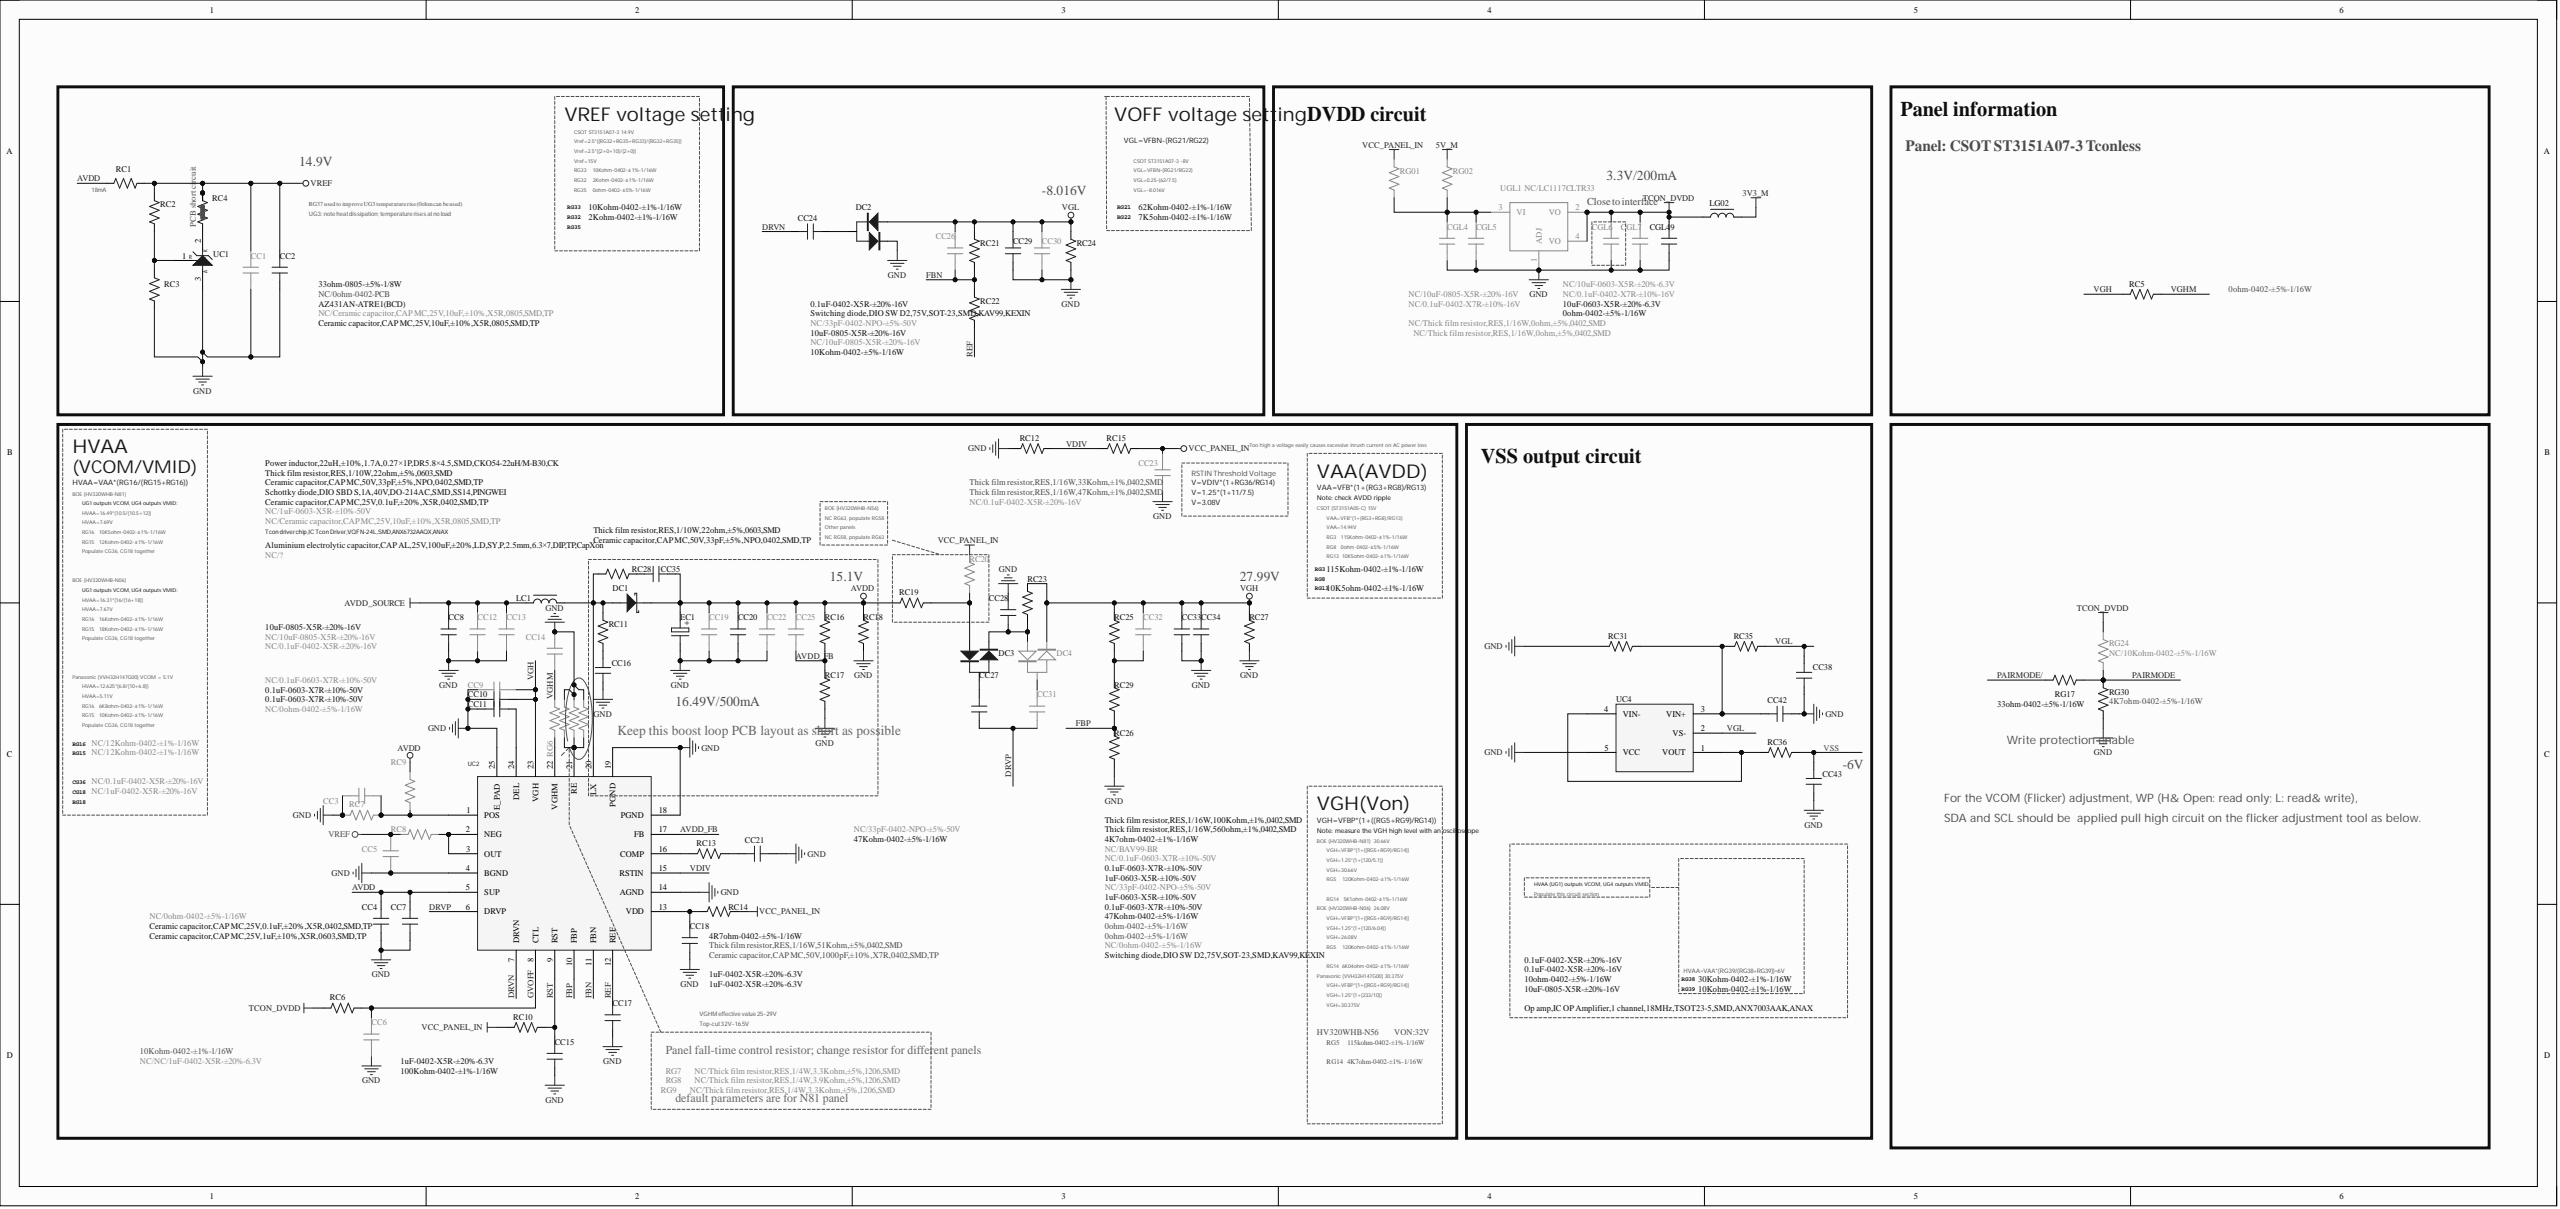Circuit board | Altium Designer | 951 parts | 509 nets | one sheet of the schematic
Parts on this sheet (reference | value | footprint):
CC1 | NC/Ceramic capacitor,CAP MC,25V,10uF,±10%,X5R,0805,SMD,TP | C0805
CC2 | Ceramic capacitor,CAP MC,25V,10uF,±10%,X5R,0805,SMD,TP | C0805
CC3 | NC/0.1uF-0402-X5R-±20%-16V | C0402
CC4 | Ceramic capacitor,CAP MC,25V,1uF,±10%,X5R,0603,SMD,TP | C0603
CC5 | NC/1uF-0402-X5R-±20%-16V | C0402
CC6 | NC/NC/1uF-0402-X5R-±20%-6.3V | C0402
CC7 | Ceramic capacitor,CAP MC,25V,0.1uF,±20%,X5R,0402,SMD,TP | C0402
CC8 | 10uF-0805-X5R-±20%-16V | C0805
CC9 | NC/0.1uF-0603-X7R-±10%-50V | C0603
CC10 | 0.1uF-0603-X7R-±10%-50V | C0603
CC11 | 0.1uF-0603-X7R-±10%-50V | C0603
CC12 | NC/10uF-0805-X5R-±20%-16V | C0805
CC13 | NC/0.1uF-0402-X5R-±20%-16V | C0402
CC14 | NC/? | C0805
CC15 | 1uF-0402-X5R-±20%-6.3V | C0402
CC16 | Ceramic capacitor,CAP MC,50V,33pF,±5%,NPO,0402,SMD,TP | C0402
CC17 | 1uF-0402-X5R-±20%-6.3V | C0402
CC18 | 1uF-0402-X5R-±20%-6.3V | C0402
CC19 | NC/Ceramic capacitor,CAP MC,25V,10uF,±10%,X5R,0805,SMD,TP | C0805
CC20 | Ceramic capacitor,CAP MC,25V,0.1uF,±20%,X5R,0402,SMD,TP | C0402
CC21 | Ceramic capacitor,CAP MC,50V,1000pF,±10%,X7R,0402,SMD,TP | C0402
CC22 | NC/1uF-0603-X5R-±10%-50V | C0603
CC23 | NC/0.1uF-0402-X5R-±20%-16V | C0402
CC24 | 0.1uF-0402-X5R-±20%-16V | C0402
CC25 | NC/33pF-0402-NPO-±5%-50V | C0402
CC26 | NC/33pF-0402-NPO-±5%-50V | C0402
CC27 | 0.1uF-0603-X7R-±10%-50V | C0603
CC28 | 1uF-0603-X5R-±10%-50V | C0603
CC29 | 10uF-0805-X5R-±20%-16V | C0805
CC30 | NC/10uF-0805-X5R-±20%-16V | C0805
CC31 | NC/0.1uF-0603-X7R-±10%-50V | C0603
CC32 | NC/33pF-0402-NPO-±5%-50V | C0402
CC33 | 1uF-0603-X5R-±10%-50V | C0603
CC34 | 0.1uF-0603-X7R-±10%-50V | C0603
CC35 | Ceramic capacitor,CAP MC,50V,33pF,±5%,NPO,0402,SMD,TP | C0402
CC38 | 0.1uF-0402-X5R-±20%-16V | C0402
CC42 | 0.1uF-0402-X5R-±20%-16V | C0402
CC43 | 10uF-0805-X5R-±20%-16V | C0805
CGL4 | NC/10uF-0805-X5R-±20%-16V | C0805
CGL5 | NC/0.1uF-0402-X7R-±10%-16V | C0402
CGL6 | NC/10uF-0603-X5R-±20%-6.3V | C0603
CGL7 | NC/0.1uF-0402-X7R-±10%-16V | C0402
CGL49 | 10uF-0603-X5R-±20%-6.3V | C0603
DC1 | Schottky diode,DIO SBD S,1A,40V,DO-214AC,SMD,SS14,PINGWEI | DIODE-S-1
DC2 | Switching diode,DIO SW D2,75V,SOT-23,SMD,KAV99,KEXIN | SO-23
DC3 | Switching diode,DIO SW D2,75V,SOT-23,SMD,KAV99,KEXIN | SO-23
DC4 | NC/BAV99-BR | SO-23
LG02 | 0ohm-0402-±5%-1/16W | L0402
RC1 | 33ohm-0805-±5%-1/8W | R0805
RC2 | 10Kohm-0402-±1%-1/16W | R0402
RC3 | 2Kohm-0402-±1%-1/16W | R0402
RC4 | NC/0ohm-0402-PCB | R0402SC
RC5 | 0ohm-0402-±5%-1/16W | R0402
RC6 | 10Kohm-0402-±1%-1/16W | R0402
RC7 | NC/12Kohm-0402-±1%-1/16W | R0402
RC8 | NC/0ohm-0402-±5%-1/16W | R0402
RC9 | NC/12Kohm-0402-±1%-1/16W | R0402
RC10 | 100Kohm-0402-±1%-1/16W | R0402
RC11 | Thick film resistor,RES,1/10W,22ohm,±5%,0603,SMD | R0603
RC12 | Thick film resistor,RES,1/16W,33Kohm,±1%,0402,SMD | R0402
RC13 | Thick film resistor,RES,1/16W,51Kohm,±5%,0402,SMD | R0402
RC14 | 4R7ohm-0402-±5%-1/16W | R0402
RC15 | Thick film resistor,RES,1/16W,47Kohm,±1%,0402,SMD | R0402
RC16 | 115Kohm-0402-±1%-1/16W | R0402
RC17 | 10K5ohm-0402-±1%-1/16W | R0402
RC18 | 47Kohm-0402-±5%-1/16W | R0402
RC19 | 0ohm-0402-±5%-1/16W | R0402
RC20 | NC/0ohm-0402-±5%-1/16W | R0402
RC21 | 62Kohm-0402-±1%-1/16W | R0402
RC22 | 7K5ohm-0402-±1%-1/16W | R0402
RC23 | 0ohm-0402-±5%-1/16W | R0402
RC24 | 10Kohm-0402-±5%-1/16W | R0402
RC25 | Thick film resistor,RES,1/16W,100Kohm,±1%,0402,SMD | R0402
RC26 | 4K7ohm-0402-±1%-1/16W | R0402
RC27 | 47Kohm-0402-±5%-1/16W | R0402
RC28 | Thick film resistor,RES,1/10W,22ohm,±5%,0603,SMD | R0603
RC29 | Thick film resistor,RES,1/16W,560ohm,±1%,0402,SMD | R0402
RC31 | 30Kohm-0402-±1%-1/16W | R0402
RC35 | 10Kohm-0402-±1%-1/16W | R0402
RC36 | 10ohm-0402-±5%-1/16W | R0402
RG01 | NC/Thick film resistor,RES,1/16W,0ohm,±5%,0402,SMD | R0402
RG02 | NC/Thick film resistor,RES,1/16W,0ohm,±5%,0402,SMD | R0402
RG6 | NC/0ohm-0402-±5%-1/16W | R0402
RG7 | NC/Thick film resistor,RES,1/4W,3.3Kohm,±5%,1206,SMD | R1206
RG8 | NC/Thick film resistor,RES,1/4W,3.9Kohm,±5%,1206,SMD | R1206
RG9 | NC/Thick film resistor,RES,1/4W,3.3Kohm,±5%,1206,SMD | R1206
RG17 | 33ohm-0402-±5%-1/16W | R0402
RG24 | NC/10Kohm-0402-±5%-1/16W | R0402
RG30 | 4K7ohm-0402-±5%-1/16W | R0402
UC1 | AZ431AN-ATRE1(BCD) | SO-23-1
UC2 | Tcon driver chip,IC Tcon Driver,VQFN-24L,SMD,ANX6732AAQX,ANAX | QFN24/0.5-5
UC4 | Op amp,IC OP Amplifier,1 channel,18MHz,TSOT23-5,SMD,ANX7003AAK,ANAX | SOT-23-5
UGL1 | NC/LC1117CLTR33 | SOT-223
Nets of these parts (net: part-pin ...):
VSS: CC43-2 RC36-2
VREF: CC1-2 CC2-2 CC5-1 RC1-2 RC2-2 RC4-2 RC4-3 RC8-1
VGL: CC26-2 CC29-1 CC30-1 CC38-1 DC2-1 RC21-2 RC24-2 RC35-2 UC4-2
VGHM: CC14-2 RC5-1 RG6-2
VGH: CC9-1 CC10-1 CC32-2 CC33-2 CC34-2 DC4-3 RC5-2 RC23-2 RC25-2 RC27-2 UC2-23
VDIV: RC12-2 RC15-1 UC2-15
VCC_PANEL_IN: CC23-2 RC10-2 RC14-2 RC15-2 RC20-1 RG01-2
TCON_DVDD: CGL6-1 CGL7-1 CGL49-1 LG02-1 RC6-2 RG24-1 UGL1-2 UGL1-4
RST: CC15-2 RC10-1 UC2-9
REF: CC17-2 RC22-1 UC2-12
PAIRMODE/: RG17-1
PAIRMODE: RG17-2 RG24-2 RG30-1
NetRG7_1: RG7-1 RG8-1 RG9-1 UC2-21
NetRG6_1: RG6-1 UC2-22
NetRC36_1: RC36-1 UC4-1 UC4-4
NetRC13_1: RC13-1 UC2-16
NetRC8_2: RC8-2 UC2-2 UC2-3
NetRC4_1: RC4-1 UC1-2
NetRC2_1: RC2-1 RC3-2 UC1-1
NetDC3_1: DC3-1 RC19-1 RC20-2
NetDC1_A: DC1-A RC11-2 RC28-2 UC2-20
NetCGL4_2: CGL4-2 CGL5-1 RG01-1 RG02-1 UGL1-3
NetCC42_1: CC42-1 RC31-2 RC35-1 UC4-3
NetCC35_2: CC35-2 RC28-1
NetCC32_1: CC32-1 RC25-1 RC29-2
NetCC31_1: CC31-1 DC4-2
NetCC28_1: CC28-1 DC3-3 DC4-1 RC23-1
NetCC27_1: CC27-1 DC3-2
NetCC24_2: CC24-2 DC2-2
NetCC21_1: CC21-1 RC13-2
NetCC18_2: CC18-2 RC14-1 UC2-13
NetCC16_2: CC16-2 RC11-1
NetCC11_1: CC11-1 UC2-24
NetCC3_1: CC3-1 RC7-1 RC9-1 UC2-1
GVOFF: CC6-2 RC6-1 UC2-8
GND: CC1-1 CC2-1 CC3-2 CC4-2 CC5-2 CC6-1 CC7-1 CC8-2 CC9-2 CC10-2 CC11-2 CC12-2 CC13-1 CC14-1 CC15-1 CC16-1 CC17-1 CC18-1 CC19-2 CC20-1 CC21-2 CC22-2 CC23-1 CC28-2 CC29-2 CC30-2 CC33-1 CC34-1 CC38-2 CC42-2 CC43-1 CGL4-1 CGL5-2 CGL6-2 CGL7-2 CGL49-2 DC2-3 RC3-1 RC7-2 RC12-1 RC17-1 RC18-1 RC24-1 RC26-1 RC27-1 RC31-1 RG7-2 RG8-2 RG9-2 RG30-2 UC1-3 UC4-5 UGL1-1 UC2-4 UC2-14 UC2-18 UC2-19
FBP: RC26-2 RC29-1 UC2-10
FBN: CC26-1 RC21-1 RC22-2 UC2-11
DRVP: CC27-2 CC31-2 UC2-6
DRVN: CC24-1 UC2-7
AVDD_SOURCE: CC8-1 CC12-1 CC13-2
AVDD_FB: CC25-1 RC16-1 RC17-2 UC2-17
AVDD: CC4-1 CC7-2 CC19-1 CC20-2 CC22-1 CC25-2 CC35-1 DC1-K RC1-1 RC9-2 RC16-2 RC18-2 RC19-2 UC2-5
5V_M: RG02-2
3V3_M: LG02-2